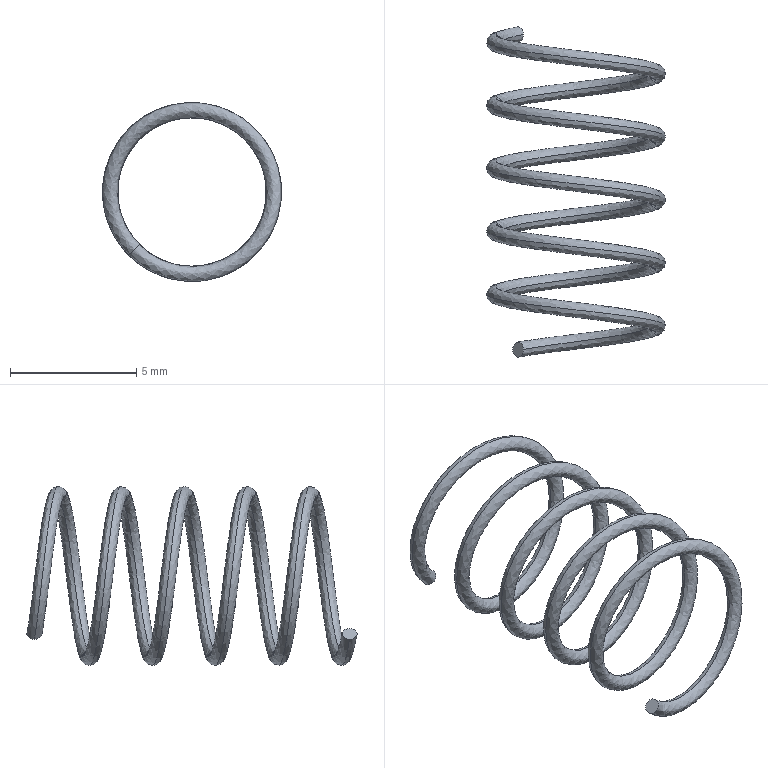Part | STEP file | Ngam kep 15 | 1 solid | 4 faces | box 7.1 x 13.1 x 7.1 mm | volume 28.863 mm3 | spline 2 | plane 2